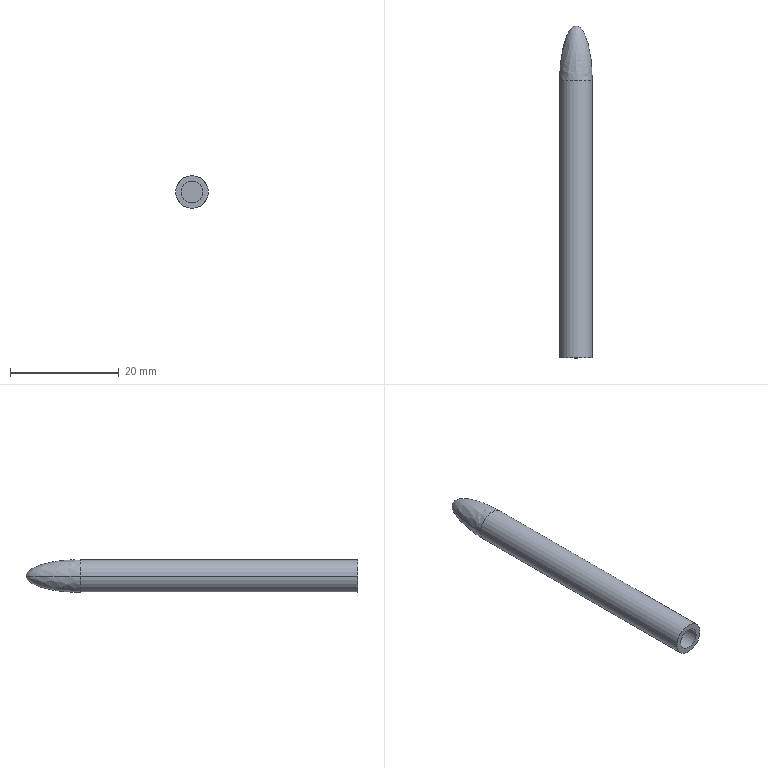Part | SolidWorks | features BaseBody 1 | 1 solid | 8 faces | box 6 x 61 x 6 mm | volume 1002 mm3 | cylinder 4 | plane 2 | spline 2 | commonest cylinder face diameters 4 x2 6 x2
STEP:
#1=CARTESIAN_POINT('',(3.,28.5,0.));
#2=VERTEX_POINT('',#1);
#3=CARTESIAN_POINT('',(-3.,28.5,0.));
#4=VERTEX_POINT('',#3);
#5=CARTESIAN_POINT('',(0.,28.5,0.));
#6=DIRECTION('',(0.,-1.,0.));
#7=DIRECTION('',(1.,0.,0.));
#8=AXIS2_PLACEMENT_3D('',#5,#6,#7);
#9=CIRCLE('',#8,3.);
#10=EDGE_CURVE('',#2,#4,#9,.T.);
#11=ORIENTED_EDGE('',*,*,#10,.T.);
#12=CARTESIAN_POINT('',(-3.,-22.5,0.));
#13=VERTEX_POINT('',#12);
#14=CARTESIAN_POINT('',(-3.,0.,0.));
#15=DIRECTION('',(0.,-1.,0.));
#16=VECTOR('',#15,1000.);
#17=LINE('',#14,#16);
#18=EDGE_CURVE('',#4,#13,#17,.T.);
#19=ORIENTED_EDGE('',*,*,#18,.T.);
#20=CARTESIAN_POINT('',(3.,-22.5,0.));
#21=VERTEX_POINT('',#20);
#22=CARTESIAN_POINT('',(0.,-22.5,0.));
#23=DIRECTION('',(0.,1.,0.));
#24=DIRECTION('',(1.,0.,0.));
#25=AXIS2_PLACEMENT_3D('',#22,#23,#24);
#26=CIRCLE('',#25,3.);
#27=EDGE_CURVE('',#13,#21,#26,.T.);
#28=ORIENTED_EDGE('',*,*,#27,.T.);
#29=CARTESIAN_POINT('',(3.,0.,0.));
#30=DIRECTION('',(0.,-1.,0.));
#31=VECTOR('',#30,1000.);
#32=LINE('',#29,#31);
#33=EDGE_CURVE('',#2,#21,#32,.T.);
#34=ORIENTED_EDGE('',*,*,#33,.F.);
#35=EDGE_LOOP('',(#11,#19,#28,#34));
#36=FACE_OUTER_BOUND('',#35,.T.);
#37=CARTESIAN_POINT('',(0.,0.,0.));
#38=DIRECTION('',(0.,-1.,0.));
#39=DIRECTION('',(1.,0.,0.));
#40=AXIS2_PLACEMENT_3D('',#37,#38,#39);
#41=CYLINDRICAL_SURFACE('',#40,3.);
#42=ADVANCED_FACE('',(#36),#41,.T.);
#43=CARTESIAN_POINT('',(-2.,27.5,0.));
#44=VERTEX_POINT('',#43);
#45=CARTESIAN_POINT('',(2.,27.5,0.));
#46=VERTEX_POINT('',#45);
#47=CARTESIAN_POINT('',(0.,27.5,0.));
#48=DIRECTION('',(0.,-1.,0.));
#49=DIRECTION('',(1.,0.,0.));
#50=AXIS2_PLACEMENT_3D('',#47,#48,#49);
#51=CIRCLE('',#50,2.);
#52=EDGE_CURVE('',#44,#46,#51,.T.);
#53=ORIENTED_EDGE('',*,*,#52,.F.);
#54=CARTESIAN_POINT('',(-2.,-22.5,0.));
#55=VERTEX_POINT('',#54);
#56=CARTESIAN_POINT('',(-2.,0.,0.));
#57=DIRECTION('',(0.,-1.,0.));
#58=VECTOR('',#57,1000.);
#59=LINE('',#56,#58);
#60=EDGE_CURVE('',#44,#55,#59,.T.);
#61=ORIENTED_EDGE('',*,*,#60,.T.);
#62=CARTESIAN_POINT('',(2.,-22.5,0.));
#63=VERTEX_POINT('',#62);
#64=CARTESIAN_POINT('',(0.,-22.5,0.));
#65=DIRECTION('',(0.,-1.,0.));
#66=DIRECTION('',(1.,0.,0.));
#67=AXIS2_PLACEMENT_3D('',#64,#65,#66);
#68=CIRCLE('',#67,2.);
#69=EDGE_CURVE('',#55,#63,#68,.T.);
#70=ORIENTED_EDGE('',*,*,#69,.T.);
#71=CARTESIAN_POINT('',(2.,0.,0.));
#72=DIRECTION('',(0.,-1.,0.));
#73=VECTOR('',#72,1000.);
#74=LINE('',#71,#73);
#75=EDGE_CURVE('',#46,#63,#74,.T.);
#76=ORIENTED_EDGE('',*,*,#75,.F.);
#77=EDGE_LOOP('',(#53,#61,#70,#76));
#78=FACE_OUTER_BOUND('',#77,.T.);
#79=CARTESIAN_POINT('',(0.,0.,0.));
#80=DIRECTION('',(0.,-1.,0.));
#81=DIRECTION('',(1.,0.,0.));
#82=AXIS2_PLACEMENT_3D('',#79,#80,#81);
#83=CYLINDRICAL_SURFACE('',#82,2.);
#84=ADVANCED_FACE('',(#78),#83,.F.);
#85=ORIENTED_EDGE('',*,*,#18,.F.);
#86=CARTESIAN_POINT('',(0.,28.5,0.));
#87=DIRECTION('',(0.,-1.,0.));
#88=DIRECTION('',(1.,0.,0.));
#89=AXIS2_PLACEMENT_3D('',#86,#87,#88);
#90=CIRCLE('',#89,3.);
#91=EDGE_CURVE('',#4,#2,#90,.T.);
#92=ORIENTED_EDGE('',*,*,#91,.T.);
#93=ORIENTED_EDGE('',*,*,#33,.T.);
#94=CARTESIAN_POINT('',(0.,-22.5,0.));
#95=DIRECTION('',(0.,1.,0.));
#96=DIRECTION('',(1.,0.,0.));
#97=AXIS2_PLACEMENT_3D('',#94,#95,#96);
#98=CIRCLE('',#97,3.);
#99=EDGE_CURVE('',#21,#13,#98,.T.);
#100=ORIENTED_EDGE('',*,*,#99,.T.);
#101=EDGE_LOOP('',(#85,#92,#93,#100));
#102=FACE_OUTER_BOUND('',#101,.T.);
#103=CARTESIAN_POINT('',(0.,0.,0.));
#104=DIRECTION('',(0.,-1.,0.));
#105=DIRECTION('',(1.,0.,0.));
#106=AXIS2_PLACEMENT_3D('',#103,#104,#105);
#107=CYLINDRICAL_SURFACE('',#106,3.);
#108=ADVANCED_FACE('',(#102),#107,.T.);
#109=ORIENTED_EDGE('',*,*,#99,.F.);
#110=ORIENTED_EDGE('',*,*,#27,.F.);
#111=EDGE_LOOP('',(#109,#110));
#112=FACE_OUTER_BOUND('',#111,.T.);
#113=CARTESIAN_POINT('',(0.,-22.5,0.));
#114=DIRECTION('',(0.,-1.,0.));
#115=DIRECTION('',(1.,0.,0.));
#116=AXIS2_PLACEMENT_3D('',#113,#114,#115);
#117=CIRCLE('',#116,2.);
#118=EDGE_CURVE('',#63,#55,#117,.T.);
#119=ORIENTED_EDGE('',*,*,#118,.F.);
#120=ORIENTED_EDGE('',*,*,#69,.F.);
#121=EDGE_LOOP('',(#119,#120));
#122=FACE_BOUND('',#121,.T.);
#123=CARTESIAN_POINT('',(-2.,-22.5,0.));
#124=DIRECTION('',(0.,1.,0.));
#125=DIRECTION('',(-1.,0.,0.));
#126=AXIS2_PLACEMENT_3D('',#123,#124,#125);
#127=PLANE('',#126);
#128=ADVANCED_FACE('',(#112,#122),#127,.F.);
#129=CARTESIAN_POINT('',(0.,38.5,0.));
#130=VERTEX_POINT('',#129);
#131=CARTESIAN_POINT('',(0.,38.5,0.));
#132=CARTESIAN_POINT('',(-1.757,38.5,0.));
#133=CARTESIAN_POINT('',(-3.,34.358,0.));
#134=CARTESIAN_POINT('',(-3.,28.5,0.));
#135=(BOUNDED_CURVE()B_SPLINE_CURVE(3,(#131,#132,#133,#134),.UNSPECIFIED.,.F.,.F.)B_SPLINE_CURVE_WITH_KNOTS((4,4),(0.,1.),.UNSPECIFIED.)CURVE()GEOMETRIC_REPRESENTATION_ITEM()RATIONAL_B_SPLINE_CURVE((1.,0.8047,0.8047,1.))REPRESENTATION_ITEM(''));
#136=EDGE_CURVE('',#130,#4,#135,.T.);
#137=ORIENTED_EDGE('',*,*,#136,.T.);
#138=ORIENTED_EDGE('',*,*,#10,.F.);
#139=CARTESIAN_POINT('',(3.,28.5,0.));
#140=CARTESIAN_POINT('',(3.,34.358,0.));
#141=CARTESIAN_POINT('',(1.757,38.5,0.));
#142=CARTESIAN_POINT('',(0.,38.5,0.));
#143=(BOUNDED_CURVE()B_SPLINE_CURVE(3,(#139,#140,#141,#142),.UNSPECIFIED.,.F.,.T.)B_SPLINE_CURVE_WITH_KNOTS((4,4),(0.,1.),.UNSPECIFIED.)CURVE()GEOMETRIC_REPRESENTATION_ITEM()RATIONAL_B_SPLINE_CURVE((1.,0.8047,0.8047,1.))REPRESENTATION_ITEM(''));
#144=EDGE_CURVE('',#2,#130,#143,.T.);
#145=ORIENTED_EDGE('',*,*,#144,.T.);
#146=EDGE_LOOP('',(#137,#138,#145));
#147=FACE_OUTER_BOUND('',#146,.T.);
#148=CARTESIAN_POINT('',(0.,38.5,0.));
#149=CARTESIAN_POINT('',(0.,38.5,0.));
#150=CARTESIAN_POINT('',(0.,38.5,0.));
#151=CARTESIAN_POINT('',(0.,38.5,0.));
#152=CARTESIAN_POINT('',(-1.757,38.5,0.));
#153=CARTESIAN_POINT('',(-1.757,38.5,3.515));
#154=CARTESIAN_POINT('',(1.757,38.5,3.515));
#155=CARTESIAN_POINT('',(1.757,38.5,0.));
#156=CARTESIAN_POINT('',(-3.,34.358,0.));
#157=CARTESIAN_POINT('',(-3.,34.358,6.));
#158=CARTESIAN_POINT('',(3.,34.358,6.));
#159=CARTESIAN_POINT('',(3.,34.358,0.));
#160=CARTESIAN_POINT('',(-3.,28.5,0.));
#161=CARTESIAN_POINT('',(-3.,28.5,6.));
#162=CARTESIAN_POINT('',(3.,28.5,6.));
#163=CARTESIAN_POINT('',(3.,28.5,0.));
#164=(BOUNDED_SURFACE()B_SPLINE_SURFACE(3,3,((#148,#149,#150,#151),(#152,#153,#154,#155),(#156,#157,#158,#159),(#160,#161,#162,#163)),.UNSPECIFIED.,.F.,.F.,.T.)B_SPLINE_SURFACE_WITH_KNOTS((4,4),(4,4),(0.,1.),(0.,1.),.UNSPECIFIED.)GEOMETRIC_REPRESENTATION_ITEM()RATIONAL_B_SPLINE_SURFACE(((1.,0.3333,0.3333,1.),(0.8047,0.2682,0.2682,0.8047),(0.8047,0.2682,0.2682,0.8047),(1.,0.3333,0.3333,1.)))REPRESENTATION_ITEM('')SURFACE());
#165=ADVANCED_FACE('',(#147),#164,.T.);
#166=ORIENTED_EDGE('',*,*,#144,.F.);
#167=ORIENTED_EDGE('',*,*,#91,.F.);
#168=ORIENTED_EDGE('',*,*,#136,.F.);
#169=EDGE_LOOP('',(#166,#167,#168));
#170=FACE_OUTER_BOUND('',#169,.T.);
#171=CARTESIAN_POINT('',(0.,38.5,0.));
#172=CARTESIAN_POINT('',(0.,38.5,0.));
#173=CARTESIAN_POINT('',(0.,38.5,0.));
#174=CARTESIAN_POINT('',(0.,38.5,0.));
#175=CARTESIAN_POINT('',(1.757,38.5,0.));
#176=CARTESIAN_POINT('',(1.757,38.5,-3.515));
#177=CARTESIAN_POINT('',(-1.757,38.5,-3.515));
#178=CARTESIAN_POINT('',(-1.757,38.5,0.));
#179=CARTESIAN_POINT('',(3.,34.358,0.));
#180=CARTESIAN_POINT('',(3.,34.358,-6.));
#181=CARTESIAN_POINT('',(-3.,34.358,-6.));
#182=CARTESIAN_POINT('',(-3.,34.358,0.));
#183=CARTESIAN_POINT('',(3.,28.5,0.));
#184=CARTESIAN_POINT('',(3.,28.5,-6.));
#185=CARTESIAN_POINT('',(-3.,28.5,-6.));
#186=CARTESIAN_POINT('',(-3.,28.5,0.));
#187=(BOUNDED_SURFACE()B_SPLINE_SURFACE(3,3,((#171,#172,#173,#174),(#175,#176,#177,#178),(#179,#180,#181,#182),(#183,#184,#185,#186)),.UNSPECIFIED.,.F.,.F.,.F.)B_SPLINE_SURFACE_WITH_KNOTS((4,4),(4,4),(0.,1.),(0.,1.),.UNSPECIFIED.)GEOMETRIC_REPRESENTATION_ITEM()RATIONAL_B_SPLINE_SURFACE(((1.,0.3333,0.3333,1.),(0.8047,0.2682,0.2682,0.8047),(0.8047,0.2682,0.2682,0.8047),(1.,0.3333,0.3333,1.)))REPRESENTATION_ITEM('')SURFACE());
#188=ADVANCED_FACE('',(#170),#187,.T.);
#189=ORIENTED_EDGE('',*,*,#60,.F.);
#190=CARTESIAN_POINT('',(0.,27.5,0.));
#191=DIRECTION('',(0.,-1.,0.));
#192=DIRECTION('',(1.,0.,0.));
#193=AXIS2_PLACEMENT_3D('',#190,#191,#192);
#194=CIRCLE('',#193,2.);
#195=EDGE_CURVE('',#46,#44,#194,.T.);
#196=ORIENTED_EDGE('',*,*,#195,.F.);
#197=ORIENTED_EDGE('',*,*,#75,.T.);
#198=ORIENTED_EDGE('',*,*,#118,.T.);
#199=EDGE_LOOP('',(#189,#196,#197,#198));
#200=FACE_OUTER_BOUND('',#199,.T.);
#201=CARTESIAN_POINT('',(0.,0.,0.));
#202=DIRECTION('',(0.,-1.,0.));
#203=DIRECTION('',(1.,0.,0.));
#204=AXIS2_PLACEMENT_3D('',#201,#202,#203);
#205=CYLINDRICAL_SURFACE('',#204,2.);
#206=ADVANCED_FACE('',(#200),#205,.F.);
#207=ORIENTED_EDGE('',*,*,#195,.T.);
#208=ORIENTED_EDGE('',*,*,#52,.T.);
#209=EDGE_LOOP('',(#207,#208));
#210=FACE_OUTER_BOUND('',#209,.T.);
#211=CARTESIAN_POINT('',(0.,27.5,0.));
#212=DIRECTION('',(0.,1.,0.));
#213=DIRECTION('',(-1.,0.,0.));
#214=AXIS2_PLACEMENT_3D('',#211,#212,#213);
#215=PLANE('',#214);
#216=ADVANCED_FACE('',(#210),#215,.F.);
#217=CLOSED_SHELL('',(#42,#84,#108,#128,#165,#188,#206,#216));
#218=MANIFOLD_SOLID_BREP('',#217);
#219=CARTESIAN_POINT('',(0.,0.,0.));
#220=DIRECTION('',(0.,0.,1.));
#221=DIRECTION('',(1.,0.,0.));
#222=AXIS2_PLACEMENT_3D('',#219,#220,#221);
#223=(LENGTH_UNIT()NAMED_UNIT(*)SI_UNIT(.MILLI.,.METRE.));
#224=UNCERTAINTY_MEASURE_WITH_UNIT(LENGTH_MEASURE(0.00001),#223,'','');
#225=(NAMED_UNIT(*)PLANE_ANGLE_UNIT()SI_UNIT($,.RADIAN.));
#226=(NAMED_UNIT(*)SI_UNIT($,.STERADIAN.)SOLID_ANGLE_UNIT());
#227=(GEOMETRIC_REPRESENTATION_CONTEXT(3)GLOBAL_UNCERTAINTY_ASSIGNED_CONTEXT((#224))GLOBAL_UNIT_ASSIGNED_CONTEXT((#223,#225,#226))REPRESENTATION_CONTEXT('',''));
#228=ADVANCED_BREP_SHAPE_REPRESENTATION('',(#218,#222),#227);